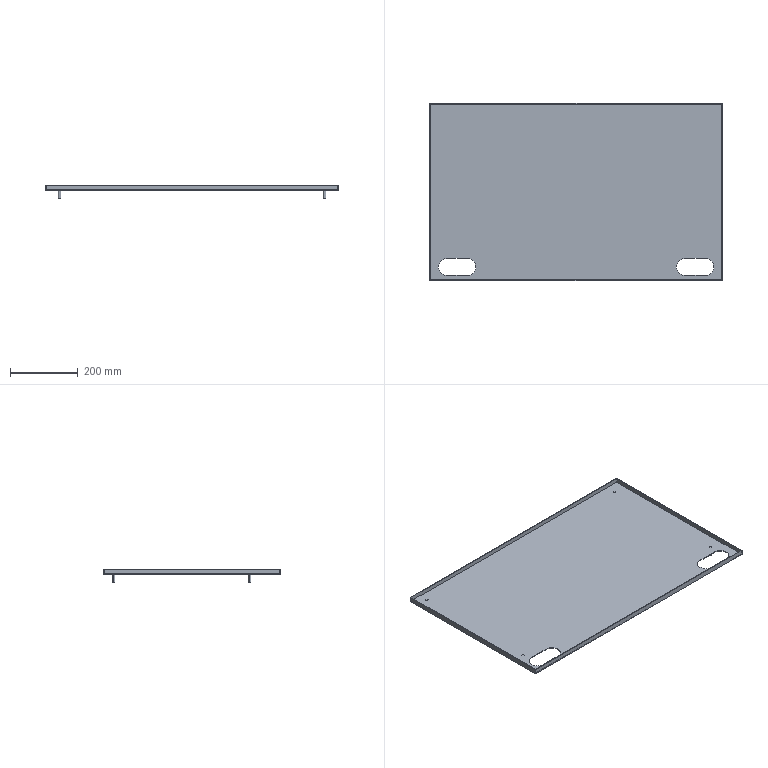Part | STEP file | 11-GYJJ-011-w111 | 1 solid | 33 faces | box 860 x 521 x 41 mm | volume 953098 mm3 | plane 19 | cylinder 14 | commonest cylinder face diameters 8 x8 50 x6
STEP:
#1=CARTESIAN_POINT('',(-394.,-169.5,-26.));
#2=VERTEX_POINT('',#1);
#3=CARTESIAN_POINT('',(-386.,-169.5,-26.));
#4=VERTEX_POINT('',#3);
#5=CARTESIAN_POINT('',(-390.,-169.5,-26.));
#6=DIRECTION('',(0.,0.,-1.));
#7=DIRECTION('',(-1.,0.,0.));
#8=AXIS2_PLACEMENT_3D('',#5,#6,#7);
#9=CIRCLE('',#8,4.);
#10=EDGE_CURVE('',#2,#4,#9,.T.);
#11=ORIENTED_EDGE('',*,*,#10,.F.);
#12=CARTESIAN_POINT('',(-394.,-169.5,0.));
#13=VERTEX_POINT('',#12);
#14=CARTESIAN_POINT('',(-394.,-169.5,-26.));
#15=DIRECTION('',(0.,0.,1.));
#16=VECTOR('',#15,1000.);
#17=LINE('',#14,#16);
#18=EDGE_CURVE('',#2,#13,#17,.T.);
#19=ORIENTED_EDGE('',*,*,#18,.T.);
#20=CARTESIAN_POINT('',(-386.,-169.5,0.));
#21=VERTEX_POINT('',#20);
#22=CARTESIAN_POINT('',(-390.,-169.5,0.));
#23=DIRECTION('',(0.,0.,-1.));
#24=DIRECTION('',(1.,0.,0.));
#25=AXIS2_PLACEMENT_3D('',#22,#23,#24);
#26=CIRCLE('',#25,4.);
#27=EDGE_CURVE('',#13,#21,#26,.T.);
#28=ORIENTED_EDGE('',*,*,#27,.T.);
#29=CARTESIAN_POINT('',(-386.,-169.5,-26.));
#30=DIRECTION('',(0.,0.,1.));
#31=VECTOR('',#30,1000.);
#32=LINE('',#29,#31);
#33=EDGE_CURVE('',#4,#21,#32,.T.);
#34=ORIENTED_EDGE('',*,*,#33,.F.);
#35=EDGE_LOOP('',(#11,#19,#28,#34));
#36=FACE_OUTER_BOUND('',#35,.T.);
#37=CARTESIAN_POINT('',(-390.,-169.5,-26.));
#38=DIRECTION('',(0.,0.,1.));
#39=DIRECTION('',(1.,0.,0.));
#40=AXIS2_PLACEMENT_3D('',#37,#38,#39);
#41=CYLINDRICAL_SURFACE('',#40,4.);
#42=ADVANCED_FACE('',(#36),#41,.T.);
#43=CARTESIAN_POINT('',(386.,-169.5,-26.));
#44=VERTEX_POINT('',#43);
#45=CARTESIAN_POINT('',(394.,-169.5,-26.));
#46=VERTEX_POINT('',#45);
#47=CARTESIAN_POINT('',(390.,-169.5,-26.));
#48=DIRECTION('',(0.,0.,-1.));
#49=DIRECTION('',(-1.,0.,0.));
#50=AXIS2_PLACEMENT_3D('',#47,#48,#49);
#51=CIRCLE('',#50,4.);
#52=EDGE_CURVE('',#44,#46,#51,.T.);
#53=ORIENTED_EDGE('',*,*,#52,.F.);
#54=CARTESIAN_POINT('',(386.,-169.5,0.));
#55=VERTEX_POINT('',#54);
#56=CARTESIAN_POINT('',(386.,-169.5,-26.));
#57=DIRECTION('',(0.,0.,1.));
#58=VECTOR('',#57,1000.);
#59=LINE('',#56,#58);
#60=EDGE_CURVE('',#44,#55,#59,.T.);
#61=ORIENTED_EDGE('',*,*,#60,.T.);
#62=CARTESIAN_POINT('',(394.,-169.5,0.));
#63=VERTEX_POINT('',#62);
#64=CARTESIAN_POINT('',(390.,-169.5,0.));
#65=DIRECTION('',(0.,0.,-1.));
#66=DIRECTION('',(1.,0.,0.));
#67=AXIS2_PLACEMENT_3D('',#64,#65,#66);
#68=CIRCLE('',#67,4.);
#69=EDGE_CURVE('',#55,#63,#68,.T.);
#70=ORIENTED_EDGE('',*,*,#69,.T.);
#71=CARTESIAN_POINT('',(394.,-169.5,-26.));
#72=DIRECTION('',(0.,0.,1.));
#73=VECTOR('',#72,1000.);
#74=LINE('',#71,#73);
#75=EDGE_CURVE('',#46,#63,#74,.T.);
#76=ORIENTED_EDGE('',*,*,#75,.F.);
#77=EDGE_LOOP('',(#53,#61,#70,#76));
#78=FACE_OUTER_BOUND('',#77,.T.);
#79=CARTESIAN_POINT('',(390.,-169.5,-26.));
#80=DIRECTION('',(0.,0.,1.));
#81=DIRECTION('',(1.,0.,0.));
#82=AXIS2_PLACEMENT_3D('',#79,#80,#81);
#83=CYLINDRICAL_SURFACE('',#82,4.);
#84=ADVANCED_FACE('',(#78),#83,.T.);
#85=CARTESIAN_POINT('',(-394.,230.5,-26.));
#86=VERTEX_POINT('',#85);
#87=CARTESIAN_POINT('',(-386.,230.5,-26.));
#88=VERTEX_POINT('',#87);
#89=CARTESIAN_POINT('',(-390.,230.5,-26.));
#90=DIRECTION('',(0.,0.,-1.));
#91=DIRECTION('',(-1.,0.,0.));
#92=AXIS2_PLACEMENT_3D('',#89,#90,#91);
#93=CIRCLE('',#92,4.);
#94=EDGE_CURVE('',#86,#88,#93,.T.);
#95=ORIENTED_EDGE('',*,*,#94,.F.);
#96=CARTESIAN_POINT('',(-394.,230.5,0.));
#97=VERTEX_POINT('',#96);
#98=CARTESIAN_POINT('',(-394.,230.5,-26.));
#99=DIRECTION('',(0.,0.,1.));
#100=VECTOR('',#99,1000.);
#101=LINE('',#98,#100);
#102=EDGE_CURVE('',#86,#97,#101,.T.);
#103=ORIENTED_EDGE('',*,*,#102,.T.);
#104=CARTESIAN_POINT('',(-386.,230.5,0.));
#105=VERTEX_POINT('',#104);
#106=CARTESIAN_POINT('',(-390.,230.5,0.));
#107=DIRECTION('',(0.,0.,-1.));
#108=DIRECTION('',(1.,0.,0.));
#109=AXIS2_PLACEMENT_3D('',#106,#107,#108);
#110=CIRCLE('',#109,4.);
#111=EDGE_CURVE('',#97,#105,#110,.T.);
#112=ORIENTED_EDGE('',*,*,#111,.T.);
#113=CARTESIAN_POINT('',(-386.,230.5,-26.));
#114=DIRECTION('',(0.,0.,1.));
#115=VECTOR('',#114,1000.);
#116=LINE('',#113,#115);
#117=EDGE_CURVE('',#88,#105,#116,.T.);
#118=ORIENTED_EDGE('',*,*,#117,.F.);
#119=EDGE_LOOP('',(#95,#103,#112,#118));
#120=FACE_OUTER_BOUND('',#119,.T.);
#121=CARTESIAN_POINT('',(-390.,230.5,-26.));
#122=DIRECTION('',(0.,0.,1.));
#123=DIRECTION('',(1.,0.,0.));
#124=AXIS2_PLACEMENT_3D('',#121,#122,#123);
#125=CYLINDRICAL_SURFACE('',#124,4.);
#126=ADVANCED_FACE('',(#120),#125,.T.);
#127=CARTESIAN_POINT('',(386.,230.5,-26.));
#128=VERTEX_POINT('',#127);
#129=CARTESIAN_POINT('',(394.,230.5,-26.));
#130=VERTEX_POINT('',#129);
#131=CARTESIAN_POINT('',(390.,230.5,-26.));
#132=DIRECTION('',(0.,0.,-1.));
#133=DIRECTION('',(-1.,0.,0.));
#134=AXIS2_PLACEMENT_3D('',#131,#132,#133);
#135=CIRCLE('',#134,4.);
#136=EDGE_CURVE('',#128,#130,#135,.T.);
#137=ORIENTED_EDGE('',*,*,#136,.F.);
#138=CARTESIAN_POINT('',(386.,230.5,0.));
#139=VERTEX_POINT('',#138);
#140=CARTESIAN_POINT('',(386.,230.5,-26.));
#141=DIRECTION('',(0.,0.,1.));
#142=VECTOR('',#141,1000.);
#143=LINE('',#140,#142);
#144=EDGE_CURVE('',#128,#139,#143,.T.);
#145=ORIENTED_EDGE('',*,*,#144,.T.);
#146=CARTESIAN_POINT('',(394.,230.5,0.));
#147=VERTEX_POINT('',#146);
#148=CARTESIAN_POINT('',(390.,230.5,0.));
#149=DIRECTION('',(0.,0.,-1.));
#150=DIRECTION('',(1.,0.,0.));
#151=AXIS2_PLACEMENT_3D('',#148,#149,#150);
#152=CIRCLE('',#151,4.);
#153=EDGE_CURVE('',#139,#147,#152,.T.);
#154=ORIENTED_EDGE('',*,*,#153,.T.);
#155=CARTESIAN_POINT('',(394.,230.5,-26.));
#156=DIRECTION('',(0.,0.,1.));
#157=VECTOR('',#156,1000.);
#158=LINE('',#155,#157);
#159=EDGE_CURVE('',#130,#147,#158,.T.);
#160=ORIENTED_EDGE('',*,*,#159,.F.);
#161=EDGE_LOOP('',(#137,#145,#154,#160));
#162=FACE_OUTER_BOUND('',#161,.T.);
#163=CARTESIAN_POINT('',(390.,230.5,-26.));
#164=DIRECTION('',(0.,0.,1.));
#165=DIRECTION('',(1.,0.,0.));
#166=AXIS2_PLACEMENT_3D('',#163,#164,#165);
#167=CYLINDRICAL_SURFACE('',#166,4.);
#168=ADVANCED_FACE('',(#162),#167,.T.);
#169=CARTESIAN_POINT('',(-405.,-220.5,2.));
#170=VERTEX_POINT('',#169);
#171=CARTESIAN_POINT('',(-380.,-195.5,2.));
#172=VERTEX_POINT('',#171);
#173=CARTESIAN_POINT('',(-380.,-220.5,2.));
#174=DIRECTION('',(0.,0.,-1.));
#175=DIRECTION('',(1.,0.,0.));
#176=AXIS2_PLACEMENT_3D('',#173,#174,#175);
#177=CIRCLE('',#176,25.);
#178=EDGE_CURVE('',#170,#172,#177,.T.);
#179=ORIENTED_EDGE('',*,*,#178,.F.);
#180=CARTESIAN_POINT('',(-405.,-220.5,0.));
#181=VERTEX_POINT('',#180);
#182=CARTESIAN_POINT('',(-405.,-220.5,10.));
#183=DIRECTION('',(0.,0.,-1.));
#184=VECTOR('',#183,1000.);
#185=LINE('',#182,#184);
#186=EDGE_CURVE('',#170,#181,#185,.T.);
#187=ORIENTED_EDGE('',*,*,#186,.T.);
#188=CARTESIAN_POINT('',(-380.,-195.5,0.));
#189=VERTEX_POINT('',#188);
#190=CARTESIAN_POINT('',(-380.,-220.5,0.));
#191=DIRECTION('',(0.,0.,1.));
#192=DIRECTION('',(1.,0.,0.));
#193=AXIS2_PLACEMENT_3D('',#190,#191,#192);
#194=CIRCLE('',#193,25.);
#195=EDGE_CURVE('',#189,#181,#194,.T.);
#196=ORIENTED_EDGE('',*,*,#195,.F.);
#197=CARTESIAN_POINT('',(-380.,-195.5,10.));
#198=DIRECTION('',(0.,0.,-1.));
#199=VECTOR('',#198,1000.);
#200=LINE('',#197,#199);
#201=EDGE_CURVE('',#172,#189,#200,.T.);
#202=ORIENTED_EDGE('',*,*,#201,.F.);
#203=EDGE_LOOP('',(#179,#187,#196,#202));
#204=FACE_OUTER_BOUND('',#203,.T.);
#205=CARTESIAN_POINT('',(-380.,-220.5,10.));
#206=DIRECTION('',(0.,0.,-1.));
#207=DIRECTION('',(-1.,0.,0.));
#208=AXIS2_PLACEMENT_3D('',#205,#206,#207);
#209=CYLINDRICAL_SURFACE('',#208,25.);
#210=ADVANCED_FACE('',(#204),#209,.F.);
#211=CARTESIAN_POINT('',(320.,-195.5,2.));
#212=VERTEX_POINT('',#211);
#213=CARTESIAN_POINT('',(295.,-220.5,2.));
#214=VERTEX_POINT('',#213);
#215=CARTESIAN_POINT('',(320.,-220.5,2.));
#216=DIRECTION('',(0.,0.,1.));
#217=DIRECTION('',(1.,0.,0.));
#218=AXIS2_PLACEMENT_3D('',#215,#216,#217);
#219=CIRCLE('',#218,25.);
#220=EDGE_CURVE('',#212,#214,#219,.T.);
#221=ORIENTED_EDGE('',*,*,#220,.T.);
#222=CARTESIAN_POINT('',(295.,-220.5,0.));
#223=VERTEX_POINT('',#222);
#224=CARTESIAN_POINT('',(295.,-220.5,10.));
#225=DIRECTION('',(0.,0.,-1.));
#226=VECTOR('',#225,1000.);
#227=LINE('',#224,#226);
#228=EDGE_CURVE('',#214,#223,#227,.T.);
#229=ORIENTED_EDGE('',*,*,#228,.T.);
#230=CARTESIAN_POINT('',(320.,-195.5,0.));
#231=VERTEX_POINT('',#230);
#232=CARTESIAN_POINT('',(320.,-220.5,0.));
#233=DIRECTION('',(0.,0.,-1.));
#234=DIRECTION('',(-1.,0.,0.));
#235=AXIS2_PLACEMENT_3D('',#232,#233,#234);
#236=CIRCLE('',#235,25.);
#237=EDGE_CURVE('',#223,#231,#236,.T.);
#238=ORIENTED_EDGE('',*,*,#237,.T.);
#239=CARTESIAN_POINT('',(320.,-195.5,10.));
#240=DIRECTION('',(0.,0.,-1.));
#241=VECTOR('',#240,1000.);
#242=LINE('',#239,#241);
#243=EDGE_CURVE('',#212,#231,#242,.T.);
#244=ORIENTED_EDGE('',*,*,#243,.F.);
#245=EDGE_LOOP('',(#221,#229,#238,#244));
#246=FACE_OUTER_BOUND('',#245,.T.);
#247=CARTESIAN_POINT('',(320.,-220.5,10.));
#248=DIRECTION('',(0.,0.,-1.));
#249=DIRECTION('',(-1.,0.,0.));
#250=AXIS2_PLACEMENT_3D('',#247,#248,#249);
#251=CYLINDRICAL_SURFACE('',#250,25.);
#252=ADVANCED_FACE('',(#246),#251,.F.);
#253=CARTESIAN_POINT('',(-390.,-169.5,0.));
#254=DIRECTION('',(0.,0.,-1.));
#255=DIRECTION('',(1.,0.,0.));
#256=AXIS2_PLACEMENT_3D('',#253,#254,#255);
#257=CIRCLE('',#256,4.);
#258=EDGE_CURVE('',#21,#13,#257,.T.);
#259=ORIENTED_EDGE('',*,*,#258,.F.);
#260=ORIENTED_EDGE('',*,*,#27,.F.);
#261=EDGE_LOOP('',(#259,#260));
#262=FACE_BOUND('',#261,.T.);
#263=CARTESIAN_POINT('',(390.,-169.5,0.));
#264=DIRECTION('',(0.,0.,-1.));
#265=DIRECTION('',(1.,0.,0.));
#266=AXIS2_PLACEMENT_3D('',#263,#264,#265);
#267=CIRCLE('',#266,4.);
#268=EDGE_CURVE('',#63,#55,#267,.T.);
#269=ORIENTED_EDGE('',*,*,#268,.F.);
#270=ORIENTED_EDGE('',*,*,#69,.F.);
#271=EDGE_LOOP('',(#269,#270));
#272=FACE_BOUND('',#271,.T.);
#273=CARTESIAN_POINT('',(-390.,230.5,0.));
#274=DIRECTION('',(0.,0.,-1.));
#275=DIRECTION('',(1.,0.,0.));
#276=AXIS2_PLACEMENT_3D('',#273,#274,#275);
#277=CIRCLE('',#276,4.);
#278=EDGE_CURVE('',#105,#97,#277,.T.);
#279=ORIENTED_EDGE('',*,*,#278,.F.);
#280=ORIENTED_EDGE('',*,*,#111,.F.);
#281=EDGE_LOOP('',(#279,#280));
#282=FACE_BOUND('',#281,.T.);
#283=CARTESIAN_POINT('',(390.,230.5,0.));
#284=DIRECTION('',(0.,0.,-1.));
#285=DIRECTION('',(1.,0.,0.));
#286=AXIS2_PLACEMENT_3D('',#283,#284,#285);
#287=CIRCLE('',#286,4.);
#288=EDGE_CURVE('',#147,#139,#287,.T.);
#289=ORIENTED_EDGE('',*,*,#288,.F.);
#290=ORIENTED_EDGE('',*,*,#153,.F.);
#291=EDGE_LOOP('',(#289,#290));
#292=FACE_BOUND('',#291,.T.);
#293=CARTESIAN_POINT('',(430.,-260.5,0.));
#294=VERTEX_POINT('',#293);
#295=CARTESIAN_POINT('',(430.,260.5,0.));
#296=VERTEX_POINT('',#295);
#297=CARTESIAN_POINT('',(430.,260.5,0.));
#298=DIRECTION('',(0.,1.,0.));
#299=VECTOR('',#298,1000.);
#300=LINE('',#297,#299);
#301=EDGE_CURVE('',#294,#296,#300,.T.);
#302=ORIENTED_EDGE('',*,*,#301,.F.);
#303=CARTESIAN_POINT('',(-430.,-260.5,0.));
#304=VERTEX_POINT('',#303);
#305=CARTESIAN_POINT('',(-430.,-260.5,0.));
#306=DIRECTION('',(1.,0.,0.));
#307=VECTOR('',#306,1000.);
#308=LINE('',#305,#307);
#309=EDGE_CURVE('',#304,#294,#308,.T.);
#310=ORIENTED_EDGE('',*,*,#309,.F.);
#311=CARTESIAN_POINT('',(-430.,260.5,0.));
#312=VERTEX_POINT('',#311);
#313=CARTESIAN_POINT('',(-430.,260.5,0.));
#314=DIRECTION('',(0.,-1.,0.));
#315=VECTOR('',#314,1000.);
#316=LINE('',#313,#315);
#317=EDGE_CURVE('',#312,#304,#316,.T.);
#318=ORIENTED_EDGE('',*,*,#317,.F.);
#319=CARTESIAN_POINT('',(-430.,260.5,0.));
#320=DIRECTION('',(-1.,0.,0.));
#321=VECTOR('',#320,1000.);
#322=LINE('',#319,#321);
#323=EDGE_CURVE('',#296,#312,#322,.T.);
#324=ORIENTED_EDGE('',*,*,#323,.F.);
#325=EDGE_LOOP('',(#302,#310,#318,#324));
#326=FACE_OUTER_BOUND('',#325,.T.);
#327=CARTESIAN_POINT('',(380.,-245.5,0.));
#328=VERTEX_POINT('',#327);
#329=CARTESIAN_POINT('',(320.,-245.5,0.));
#330=VERTEX_POINT('',#329);
#331=CARTESIAN_POINT('',(380.,-245.5,0.));
#332=DIRECTION('',(-1.,0.,0.));
#333=VECTOR('',#332,1000.);
#334=LINE('',#331,#333);
#335=EDGE_CURVE('',#328,#330,#334,.T.);
#336=ORIENTED_EDGE('',*,*,#335,.F.);
#337=CARTESIAN_POINT('',(380.,-195.5,0.));
#338=VERTEX_POINT('',#337);
#339=CARTESIAN_POINT('',(380.,-220.5,0.));
#340=DIRECTION('',(0.,0.,-1.));
#341=DIRECTION('',(-1.,0.,0.));
#342=AXIS2_PLACEMENT_3D('',#339,#340,#341);
#343=CIRCLE('',#342,25.);
#344=EDGE_CURVE('',#338,#328,#343,.T.);
#345=ORIENTED_EDGE('',*,*,#344,.F.);
#346=CARTESIAN_POINT('',(380.,-195.5,0.));
#347=DIRECTION('',(1.,0.,0.));
#348=VECTOR('',#347,1000.);
#349=LINE('',#346,#348);
#350=EDGE_CURVE('',#231,#338,#349,.T.);
#351=ORIENTED_EDGE('',*,*,#350,.F.);
#352=ORIENTED_EDGE('',*,*,#237,.F.);
#353=CARTESIAN_POINT('',(320.,-220.5,0.));
#354=DIRECTION('',(0.,0.,-1.));
#355=DIRECTION('',(-1.,0.,0.));
#356=AXIS2_PLACEMENT_3D('',#353,#354,#355);
#357=CIRCLE('',#356,25.);
#358=EDGE_CURVE('',#330,#223,#357,.T.);
#359=ORIENTED_EDGE('',*,*,#358,.F.);
#360=EDGE_LOOP('',(#336,#345,#351,#352,#359));
#361=FACE_BOUND('',#360,.T.);
#362=ORIENTED_EDGE('',*,*,#195,.T.);
#363=CARTESIAN_POINT('',(-380.,-245.5,0.));
#364=VERTEX_POINT('',#363);
#365=CARTESIAN_POINT('',(-380.,-220.5,0.));
#366=DIRECTION('',(0.,0.,1.));
#367=DIRECTION('',(1.,0.,0.));
#368=AXIS2_PLACEMENT_3D('',#365,#366,#367);
#369=CIRCLE('',#368,25.);
#370=EDGE_CURVE('',#181,#364,#369,.T.);
#371=ORIENTED_EDGE('',*,*,#370,.T.);
#372=CARTESIAN_POINT('',(-320.,-245.5,0.));
#373=VERTEX_POINT('',#372);
#374=CARTESIAN_POINT('',(-380.,-245.5,0.));
#375=DIRECTION('',(1.,0.,0.));
#376=VECTOR('',#375,1000.);
#377=LINE('',#374,#376);
#378=EDGE_CURVE('',#364,#373,#377,.T.);
#379=ORIENTED_EDGE('',*,*,#378,.T.);
#380=CARTESIAN_POINT('',(-320.,-195.5,0.));
#381=VERTEX_POINT('',#380);
#382=CARTESIAN_POINT('',(-320.,-220.5,0.));
#383=DIRECTION('',(0.,0.,1.));
#384=DIRECTION('',(1.,0.,0.));
#385=AXIS2_PLACEMENT_3D('',#382,#383,#384);
#386=CIRCLE('',#385,25.);
#387=EDGE_CURVE('',#373,#381,#386,.T.);
#388=ORIENTED_EDGE('',*,*,#387,.T.);
#389=CARTESIAN_POINT('',(-380.,-195.5,0.));
#390=DIRECTION('',(-1.,0.,0.));
#391=VECTOR('',#390,1000.);
#392=LINE('',#389,#391);
#393=EDGE_CURVE('',#381,#189,#392,.T.);
#394=ORIENTED_EDGE('',*,*,#393,.T.);
#395=EDGE_LOOP('',(#362,#371,#379,#388,#394));
#396=FACE_BOUND('',#395,.T.);
#397=CARTESIAN_POINT('',(0.,0.,0.));
#398=DIRECTION('',(0.,0.,1.));
#399=DIRECTION('',(1.,0.,0.));
#400=AXIS2_PLACEMENT_3D('',#397,#398,#399);
#401=PLANE('',#400);
#402=ADVANCED_FACE('',(#262,#272,#282,#292,#326,#361,#396),#401,.F.);
#403=CARTESIAN_POINT('',(380.,-245.5,2.));
#404=VERTEX_POINT('',#403);
#405=CARTESIAN_POINT('',(380.,-195.5,2.));
#406=VERTEX_POINT('',#405);
#407=CARTESIAN_POINT('',(380.,-220.5,2.));
#408=DIRECTION('',(0.,0.,1.));
#409=DIRECTION('',(1.,0.,0.));
#410=AXIS2_PLACEMENT_3D('',#407,#408,#409);
#411=CIRCLE('',#410,25.);
#412=EDGE_CURVE('',#404,#406,#411,.T.);
#413=ORIENTED_EDGE('',*,*,#412,.F.);
#414=CARTESIAN_POINT('',(320.,-245.5,2.));
#415=VERTEX_POINT('',#414);
#416=CARTESIAN_POINT('',(0.,-245.5,2.));
#417=DIRECTION('',(1.,0.,0.));
#418=VECTOR('',#417,1000.);
#419=LINE('',#416,#418);
#420=EDGE_CURVE('',#415,#404,#419,.T.);
#421=ORIENTED_EDGE('',*,*,#420,.F.);
#422=CARTESIAN_POINT('',(320.,-220.5,2.));
#423=DIRECTION('',(0.,0.,1.));
#424=DIRECTION('',(1.,0.,0.));
#425=AXIS2_PLACEMENT_3D('',#422,#423,#424);
#426=CIRCLE('',#425,25.);
#427=EDGE_CURVE('',#214,#415,#426,.T.);
#428=ORIENTED_EDGE('',*,*,#427,.F.);
#429=ORIENTED_EDGE('',*,*,#220,.F.);
#430=CARTESIAN_POINT('',(0.,-195.5,2.));
#431=DIRECTION('',(-1.,0.,0.));
#432=VECTOR('',#431,1000.);
#433=LINE('',#430,#432);
#434=EDGE_CURVE('',#406,#212,#433,.T.);
#435=ORIENTED_EDGE('',*,*,#434,.F.);
#436=EDGE_LOOP('',(#413,#421,#428,#429,#435));
#437=FACE_BOUND('',#436,.T.);
#438=CARTESIAN_POINT('',(428.,-258.5,2.));
#439=VERTEX_POINT('',#438);
#440=CARTESIAN_POINT('',(428.,258.5,2.));
#441=VERTEX_POINT('',#440);
#442=CARTESIAN_POINT('',(428.,260.5,2.));
#443=DIRECTION('',(0.,1.,0.));
#444=VECTOR('',#443,1000.);
#445=LINE('',#442,#444);
#446=EDGE_CURVE('',#439,#441,#445,.T.);
#447=ORIENTED_EDGE('',*,*,#446,.T.);
#448=CARTESIAN_POINT('',(-428.,258.5,2.));
#449=VERTEX_POINT('',#448);
#450=CARTESIAN_POINT('',(-430.,258.5,2.));
#451=DIRECTION('',(-1.,0.,0.));
#452=VECTOR('',#451,1000.);
#453=LINE('',#450,#452);
#454=EDGE_CURVE('',#441,#449,#453,.T.);
#455=ORIENTED_EDGE('',*,*,#454,.T.);
#456=CARTESIAN_POINT('',(-428.,-258.5,2.));
#457=VERTEX_POINT('',#456);
#458=CARTESIAN_POINT('',(-428.,260.5,2.));
#459=DIRECTION('',(0.,-1.,0.));
#460=VECTOR('',#459,1000.);
#461=LINE('',#458,#460);
#462=EDGE_CURVE('',#449,#457,#461,.T.);
#463=ORIENTED_EDGE('',*,*,#462,.T.);
#464=CARTESIAN_POINT('',(-430.,-258.5,2.));
#465=DIRECTION('',(1.,0.,0.));
#466=VECTOR('',#465,1000.);
#467=LINE('',#464,#466);
#468=EDGE_CURVE('',#457,#439,#467,.T.);
#469=ORIENTED_EDGE('',*,*,#468,.T.);
#470=EDGE_LOOP('',(#447,#455,#463,#469));
#471=FACE_OUTER_BOUND('',#470,.T.);
#472=CARTESIAN_POINT('',(-320.,-245.5,2.));
#473=VERTEX_POINT('',#472);
#474=CARTESIAN_POINT('',(-380.,-245.5,2.));
#475=VERTEX_POINT('',#474);
#476=CARTESIAN_POINT('',(0.,-245.5,2.));
#477=DIRECTION('',(-1.,0.,0.));
#478=VECTOR('',#477,1000.);
#479=LINE('',#476,#478);
#480=EDGE_CURVE('',#473,#475,#479,.T.);
#481=ORIENTED_EDGE('',*,*,#480,.T.);
#482=CARTESIAN_POINT('',(-380.,-220.5,2.));
#483=DIRECTION('',(0.,0.,-1.));
#484=DIRECTION('',(1.,0.,0.));
#485=AXIS2_PLACEMENT_3D('',#482,#483,#484);
#486=CIRCLE('',#485,25.);
#487=EDGE_CURVE('',#475,#170,#486,.T.);
#488=ORIENTED_EDGE('',*,*,#487,.T.);
#489=ORIENTED_EDGE('',*,*,#178,.T.);
#490=CARTESIAN_POINT('',(-320.,-195.5,2.));
#491=VERTEX_POINT('',#490);
#492=CARTESIAN_POINT('',(0.,-195.5,2.));
#493=DIRECTION('',(1.,0.,0.));
#494=VECTOR('',#493,1000.);
#495=LINE('',#492,#494);
#496=EDGE_CURVE('',#172,#491,#495,.T.);
#497=ORIENTED_EDGE('',*,*,#496,.T.);
#498=CARTESIAN_POINT('',(-320.,-220.5,2.));
#499=DIRECTION('',(0.,0.,-1.));
#500=DIRECTION('',(1.,0.,0.));
#501=AXIS2_PLACEMENT_3D('',#498,#499,#500);
#502=CIRCLE('',#501,25.);
#503=EDGE_CURVE('',#491,#473,#502,.T.);
#504=ORIENTED_EDGE('',*,*,#503,.T.);
#505=EDGE_LOOP('',(#481,#488,#489,#497,#504));
#506=FACE_BOUND('',#505,.T.);
#507=CARTESIAN_POINT('',(0.,0.,2.));
#508=DIRECTION('',(0.,0.,1.));
#509=DIRECTION('',(1.,0.,0.));
#510=AXIS2_PLACEMENT_3D('',#507,#508,#509);
#511=PLANE('',#510);
#512=ADVANCED_FACE('',(#437,#471,#506),#511,.T.);
#513=ORIENTED_EDGE('',*,*,#301,.T.);
#514=CARTESIAN_POINT('',(430.,260.5,15.));
#515=VERTEX_POINT('',#514);
#516=CARTESIAN_POINT('',(430.,260.5,15.));
#517=DIRECTION('',(0.,0.,-1.));
#518=VECTOR('',#517,1000.);
#519=LINE('',#516,#518);
#520=EDGE_CURVE('',#515,#296,#519,.T.);
#521=ORIENTED_EDGE('',*,*,#520,.F.);
#522=CARTESIAN_POINT('',(430.,-260.5,15.));
#523=VERTEX_POINT('',#522);
#524=CARTESIAN_POINT('',(430.,260.5,15.));
#525=DIRECTION('',(0.,1.,0.));
#526=VECTOR('',#525,1000.);
#527=LINE('',#524,#526);
#528=EDGE_CURVE('',#523,#515,#527,.T.);
#529=ORIENTED_EDGE('',*,*,#528,.F.);
#530=CARTESIAN_POINT('',(430.,-260.5,15.));
#531=DIRECTION('',(0.,0.,-1.));
#532=VECTOR('',#531,1000.);
#533=LINE('',#530,#532);
#534=EDGE_CURVE('',#523,#294,#533,.T.);
#535=ORIENTED_EDGE('',*,*,#534,.T.);
#536=EDGE_LOOP('',(#513,#521,#529,#535));
#537=FACE_OUTER_BOUND('',#536,.T.);
#538=CARTESIAN_POINT('',(430.,260.5,15.));
#539=DIRECTION('',(-1.,0.,0.));
#540=DIRECTION('',(0.,-1.,0.));
#541=AXIS2_PLACEMENT_3D('',#538,#539,#540);
#542=PLANE('',#541);
#543=ADVANCED_FACE('',(#537),#542,.F.);
#544=ORIENTED_EDGE('',*,*,#323,.T.);
#545=CARTESIAN_POINT('',(-430.,260.5,15.));
#546=VERTEX_POINT('',#545);
#547=CARTESIAN_POINT('',(-430.,260.5,15.));
#548=DIRECTION('',(0.,0.,-1.));
#549=VECTOR('',#548,1000.);
#550=LINE('',#547,#549);
#551=EDGE_CURVE('',#546,#312,#550,.T.);
#552=ORIENTED_EDGE('',*,*,#551,.F.);
#553=CARTESIAN_POINT('',(-430.,260.5,15.));
#554=DIRECTION('',(-1.,0.,0.));
#555=VECTOR('',#554,1000.);
#556=LINE('',#553,#555);
#557=EDGE_CURVE('',#515,#546,#556,.T.);
#558=ORIENTED_EDGE('',*,*,#557,.F.);
#559=ORIENTED_EDGE('',*,*,#520,.T.);
#560=EDGE_LOOP('',(#544,#552,#558,#559));
#561=FACE_OUTER_BOUND('',#560,.T.);
#562=CARTESIAN_POINT('',(-430.,260.5,15.));
#563=DIRECTION('',(0.,-1.,0.));
#564=DIRECTION('',(0.,0.,-1.));
#565=AXIS2_PLACEMENT_3D('',#562,#563,#564);
#566=PLANE('',#565);
#567=ADVANCED_FACE('',(#561),#566,.F.);
#568=ORIENTED_EDGE('',*,*,#317,.T.);
#569=CARTESIAN_POINT('',(-430.,-260.5,15.));
#570=VERTEX_POINT('',#569);
#571=CARTESIAN_POINT('',(-430.,-260.5,15.));
#572=DIRECTION('',(0.,0.,-1.));
#573=VECTOR('',#572,1000.);
#574=LINE('',#571,#573);
#575=EDGE_CURVE('',#570,#304,#574,.T.);
#576=ORIENTED_EDGE('',*,*,#575,.F.);
#577=CARTESIAN_POINT('',(-430.,260.5,15.));
#578=DIRECTION('',(0.,-1.,0.));
#579=VECTOR('',#578,1000.);
#580=LINE('',#577,#579);
#581=EDGE_CURVE('',#546,#570,#580,.T.);
#582=ORIENTED_EDGE('',*,*,#581,.F.);
#583=ORIENTED_EDGE('',*,*,#551,.T.);
#584=EDGE_LOOP('',(#568,#576,#582,#583));
#585=FACE_OUTER_BOUND('',#584,.T.);
#586=CARTESIAN_POINT('',(-430.,260.5,15.));
#587=DIRECTION('',(1.,0.,0.));
#588=DIRECTION('',(0.,0.,-1.));
#589=AXIS2_PLACEMENT_3D('',#586,#587,#588);
#590=PLANE('',#589);
#591=ADVANCED_FACE('',(#585),#590,.F.);
#592=ORIENTED_EDGE('',*,*,#309,.T.);
#593=ORIENTED_EDGE('',*,*,#534,.F.);
#594=CARTESIAN_POINT('',(-430.,-260.5,15.));
#595=DIRECTION('',(1.,0.,0.));
#596=VECTOR('',#595,1000.);
#597=LINE('',#594,#596);
#598=EDGE_CURVE('',#570,#523,#597,.T.);
#599=ORIENTED_EDGE('',*,*,#598,.F.);
#600=ORIENTED_EDGE('',*,*,#575,.T.);
#601=EDGE_LOOP('',(#592,#593,#599,#600));
#602=FACE_OUTER_BOUND('',#601,.T.);
#603=CARTESIAN_POINT('',(-430.,-260.5,15.));
#604=DIRECTION('',(0.,1.,0.));
#605=DIRECTION('',(0.,0.,1.));
#606=AXIS2_PLACEMENT_3D('',#603,#604,#605);
#607=PLANE('',#606);
#608=ADVANCED_FACE('',(#602),#607,.F.);
#609=CARTESIAN_POINT('',(428.,-258.5,15.));
#610=VERTEX_POINT('',#609);
#611=CARTESIAN_POINT('',(428.,258.5,15.));
#612=VERTEX_POINT('',#611);
#613=CARTESIAN_POINT('',(428.,260.5,15.));
#614=DIRECTION('',(0.,1.,0.));
#615=VECTOR('',#614,1000.);
#616=LINE('',#613,#615);
#617=EDGE_CURVE('',#610,#612,#616,.T.);
#618=ORIENTED_EDGE('',*,*,#617,.F.);
#619=CARTESIAN_POINT('',(-428.,-258.5,15.));
#620=VERTEX_POINT('',#619);
#621=CARTESIAN_POINT('',(-430.,-258.5,15.));
#622=DIRECTION('',(1.,0.,0.));
#623=VECTOR('',#622,1000.);
#624=LINE('',#621,#623);
#625=EDGE_CURVE('',#620,#610,#624,.T.);
#626=ORIENTED_EDGE('',*,*,#625,.F.);
#627=CARTESIAN_POINT('',(-428.,258.5,15.));
#628=VERTEX_POINT('',#627);
#629=CARTESIAN_POINT('',(-428.,260.5,15.));
#630=DIRECTION('',(0.,-1.,0.));
#631=VECTOR('',#630,1000.);
#632=LINE('',#629,#631);
#633=EDGE_CURVE('',#628,#620,#632,.T.);
#634=ORIENTED_EDGE('',*,*,#633,.F.);
#635=CARTESIAN_POINT('',(-430.,258.5,15.));
#636=DIRECTION('',(-1.,0.,0.));
#637=VECTOR('',#636,1000.);
#638=LINE('',#635,#637);
#639=EDGE_CURVE('',#612,#628,#638,.T.);
#640=ORIENTED_EDGE('',*,*,#639,.F.);
#641=EDGE_LOOP('',(#618,#626,#634,#640));
#642=FACE_BOUND('',#641,.T.);
#643=ORIENTED_EDGE('',*,*,#528,.T.);
#644=ORIENTED_EDGE('',*,*,#557,.T.);
#645=ORIENTED_EDGE('',*,*,#581,.T.);
#646=ORIENTED_EDGE('',*,*,#598,.T.);
#647=EDGE_LOOP('',(#643,#644,#645,#646));
#648=FACE_OUTER_BOUND('',#647,.T.);
#649=CARTESIAN_POINT('',(0.,0.,15.));
#650=DIRECTION('',(0.,0.,1.));
#651=DIRECTION('',(1.,0.,0.));
#652=AXIS2_PLACEMENT_3D('',#649,#650,#651);
#653=PLANE('',#652);
#654=ADVANCED_FACE('',(#642,#648),#653,.T.);
#655=ORIENTED_EDGE('',*,*,#446,.F.);
#656=CARTESIAN_POINT('',(428.,-258.5,15.));
#657=DIRECTION('',(0.,0.,-1.));
#658=VECTOR('',#657,1000.);
#659=LINE('',#656,#658);
#660=EDGE_CURVE('',#610,#439,#659,.T.);
#661=ORIENTED_EDGE('',*,*,#660,.F.);
#662=ORIENTED_EDGE('',*,*,#617,.T.);
#663=CARTESIAN_POINT('',(428.,258.5,15.));
#664=DIRECTION('',(0.,0.,-1.));
#665=VECTOR('',#664,1000.);
#666=LINE('',#663,#665);
#667=EDGE_CURVE('',#612,#441,#666,.T.);
#668=ORIENTED_EDGE('',*,*,#667,.T.);
#669=EDGE_LOOP('',(#655,#661,#662,#668));
#670=FACE_OUTER_BOUND('',#669,.T.);
#671=CARTESIAN_POINT('',(428.,260.5,15.));
#672=DIRECTION('',(-1.,0.,0.));
#673=DIRECTION('',(0.,-1.,0.));
#674=AXIS2_PLACEMENT_3D('',#671,#672,#673);
#675=PLANE('',#674);
#676=ADVANCED_FACE('',(#670),#675,.T.);
#677=ORIENTED_EDGE('',*,*,#454,.F.);
#678=ORIENTED_EDGE('',*,*,#667,.F.);
#679=ORIENTED_EDGE('',*,*,#639,.T.);
#680=CARTESIAN_POINT('',(-428.,258.5,15.));
#681=DIRECTION('',(0.,0.,-1.));
#682=VECTOR('',#681,1000.);
#683=LINE('',#680,#682);
#684=EDGE_CURVE('',#628,#449,#683,.T.);
#685=ORIENTED_EDGE('',*,*,#684,.T.);
#686=EDGE_LOOP('',(#677,#678,#679,#685));
#687=FACE_OUTER_BOUND('',#686,.T.);
#688=CARTESIAN_POINT('',(-430.,258.5,15.));
#689=DIRECTION('',(0.,-1.,0.));
#690=DIRECTION('',(0.,0.,-1.));
#691=AXIS2_PLACEMENT_3D('',#688,#689,#690);
#692=PLANE('',#691);
#693=ADVANCED_FACE('',(#687),#692,.T.);
#694=ORIENTED_EDGE('',*,*,#462,.F.);
#695=ORIENTED_EDGE('',*,*,#684,.F.);
#696=ORIENTED_EDGE('',*,*,#633,.T.);
#697=CARTESIAN_POINT('',(-428.,-258.5,15.));
#698=DIRECTION('',(0.,0.,-1.));
#699=VECTOR('',#698,1000.);
#700=LINE('',#697,#699);
#701=EDGE_CURVE('',#620,#457,#700,.T.);
#702=ORIENTED_EDGE('',*,*,#701,.T.);
#703=EDGE_LOOP('',(#694,#695,#696,#702));
#704=FACE_OUTER_BOUND('',#703,.T.);
#705=CARTESIAN_POINT('',(-428.,260.5,15.));
#706=DIRECTION('',(1.,0.,0.));
#707=DIRECTION('',(0.,0.,-1.));
#708=AXIS2_PLACEMENT_3D('',#705,#706,#707);
#709=PLANE('',#708);
#710=ADVANCED_FACE('',(#704),#709,.T.);
#711=ORIENTED_EDGE('',*,*,#468,.F.);
#712=ORIENTED_EDGE('',*,*,#701,.F.);
#713=ORIENTED_EDGE('',*,*,#625,.T.);
#714=ORIENTED_EDGE('',*,*,#660,.T.);
#715=EDGE_LOOP('',(#711,#712,#713,#714));
#716=FACE_OUTER_BOUND('',#715,.T.);
#717=CARTESIAN_POINT('',(-430.,-258.5,15.));
#718=DIRECTION('',(0.,1.,0.));
#719=DIRECTION('',(0.,0.,1.));
#720=AXIS2_PLACEMENT_3D('',#717,#718,#719);
#721=PLANE('',#720);
#722=ADVANCED_FACE('',(#716),#721,.T.);
#723=ORIENTED_EDGE('',*,*,#412,.T.);
#724=CARTESIAN_POINT('',(380.,-195.5,10.));
#725=DIRECTION('',(0.,0.,-1.));
#726=VECTOR('',#725,1000.);
#727=LINE('',#724,#726);
#728=EDGE_CURVE('',#406,#338,#727,.T.);
#729=ORIENTED_EDGE('',*,*,#728,.T.);
#730=ORIENTED_EDGE('',*,*,#344,.T.);
#731=CARTESIAN_POINT('',(380.,-245.5,10.));
#732=DIRECTION('',(0.,0.,-1.));
#733=VECTOR('',#732,1000.);
#734=LINE('',#731,#733);
#735=EDGE_CURVE('',#404,#328,#734,.T.);
#736=ORIENTED_EDGE('',*,*,#735,.F.);
#737=EDGE_LOOP('',(#723,#729,#730,#736));
#738=FACE_OUTER_BOUND('',#737,.T.);
#739=CARTESIAN_POINT('',(380.,-220.5,10.));
#740=DIRECTION('',(0.,0.,-1.));
#741=DIRECTION('',(-1.,0.,0.));
#742=AXIS2_PLACEMENT_3D('',#739,#740,#741);
#743=CYLINDRICAL_SURFACE('',#742,25.);
#744=ADVANCED_FACE('',(#738),#743,.F.);
#745=ORIENTED_EDGE('',*,*,#434,.T.);
#746=ORIENTED_EDGE('',*,*,#243,.T.);
#747=ORIENTED_EDGE('',*,*,#350,.T.);
#748=ORIENTED_EDGE('',*,*,#728,.F.);
#749=EDGE_LOOP('',(#745,#746,#747,#748));
#750=FACE_OUTER_BOUND('',#749,.T.);
#751=CARTESIAN_POINT('',(380.,-195.5,10.));
#752=DIRECTION('',(0.,1.,0.));
#753=DIRECTION('',(0.,0.,1.));
#754=AXIS2_PLACEMENT_3D('',#751,#752,#753);
#755=PLANE('',#754);
#756=ADVANCED_FACE('',(#750),#755,.F.);
#757=ORIENTED_EDGE('',*,*,#228,.F.);
#758=ORIENTED_EDGE('',*,*,#427,.T.);
#759=CARTESIAN_POINT('',(320.,-245.5,10.));
#760=DIRECTION('',(0.,0.,-1.));
#761=VECTOR('',#760,1000.);
#762=LINE('',#759,#761);
#763=EDGE_CURVE('',#415,#330,#762,.T.);
#764=ORIENTED_EDGE('',*,*,#763,.T.);
#765=ORIENTED_EDGE('',*,*,#358,.T.);
#766=EDGE_LOOP('',(#757,#758,#764,#765));
#767=FACE_OUTER_BOUND('',#766,.T.);
#768=CARTESIAN_POINT('',(320.,-220.5,10.));
#769=DIRECTION('',(0.,0.,-1.));
#770=DIRECTION('',(-1.,0.,0.));
#771=AXIS2_PLACEMENT_3D('',#768,#769,#770);
#772=CYLINDRICAL_SURFACE('',#771,25.);
#773=ADVANCED_FACE('',(#767),#772,.F.);
#774=ORIENTED_EDGE('',*,*,#420,.T.);
#775=ORIENTED_EDGE('',*,*,#735,.T.);
#776=ORIENTED_EDGE('',*,*,#335,.T.);
#777=ORIENTED_EDGE('',*,*,#763,.F.);
#778=EDGE_LOOP('',(#774,#775,#776,#777));
#779=FACE_OUTER_BOUND('',#778,.T.);
#780=CARTESIAN_POINT('',(380.,-245.5,10.));
#781=DIRECTION('',(0.,-1.,0.));
#782=DIRECTION('',(0.,0.,-1.));
#783=AXIS2_PLACEMENT_3D('',#780,#781,#782);
#784=PLANE('',#783);
#785=ADVANCED_FACE('',(#779),#784,.F.);
#786=ORIENTED_EDGE('',*,*,#186,.F.);
#787=ORIENTED_EDGE('',*,*,#487,.F.);
#788=CARTESIAN_POINT('',(-380.,-245.5,10.));
#789=DIRECTION('',(0.,0.,-1.));
#790=VECTOR('',#789,1000.);
#791=LINE('',#788,#790);
#792=EDGE_CURVE('',#475,#364,#791,.T.);
#793=ORIENTED_EDGE('',*,*,#792,.T.);
#794=ORIENTED_EDGE('',*,*,#370,.F.);
#795=EDGE_LOOP('',(#786,#787,#793,#794));
#796=FACE_OUTER_BOUND('',#795,.T.);
#797=CARTESIAN_POINT('',(-380.,-220.5,10.));
#798=DIRECTION('',(0.,0.,-1.));
#799=DIRECTION('',(-1.,0.,0.));
#800=AXIS2_PLACEMENT_3D('',#797,#798,#799);
#801=CYLINDRICAL_SURFACE('',#800,25.);
#802=ADVANCED_FACE('',(#796),#801,.F.);
#803=CARTESIAN_POINT('',(-320.,-245.5,10.));
#804=DIRECTION('',(0.,0.,-1.));
#805=VECTOR('',#804,1000.);
#806=LINE('',#803,#805);
#807=EDGE_CURVE('',#473,#373,#806,.T.);
#808=ORIENTED_EDGE('',*,*,#807,.T.);
#809=ORIENTED_EDGE('',*,*,#378,.F.);
#810=ORIENTED_EDGE('',*,*,#792,.F.);
#811=ORIENTED_EDGE('',*,*,#480,.F.);
#812=EDGE_LOOP('',(#808,#809,#810,#811));
#813=FACE_OUTER_BOUND('',#812,.T.);
#814=CARTESIAN_POINT('',(-380.,-245.5,10.));
#815=DIRECTION('',(0.,1.,0.));
#816=DIRECTION('',(-1.,0.,0.));
#817=AXIS2_PLACEMENT_3D('',#814,#815,#816);
#818=PLANE('',#817);
#819=ADVANCED_FACE('',(#813),#818,.T.);
#820=CARTESIAN_POINT('',(-320.,-195.5,10.));
#821=DIRECTION('',(0.,0.,-1.));
#822=VECTOR('',#821,1000.);
#823=LINE('',#820,#822);
#824=EDGE_CURVE('',#491,#381,#823,.T.);
#825=ORIENTED_EDGE('',*,*,#824,.T.);
#826=ORIENTED_EDGE('',*,*,#387,.F.);
#827=ORIENTED_EDGE('',*,*,#807,.F.);
#828=ORIENTED_EDGE('',*,*,#503,.F.);
#829=EDGE_LOOP('',(#825,#826,#827,#828));
#830=FACE_OUTER_BOUND('',#829,.T.);
#831=CARTESIAN_POINT('',(-320.,-220.5,10.));
#832=DIRECTION('',(0.,0.,-1.));
#833=DIRECTION('',(-1.,0.,0.));
#834=AXIS2_PLACEMENT_3D('',#831,#832,#833);
#835=CYLINDRICAL_SURFACE('',#834,25.);
#836=ADVANCED_FACE('',(#830),#835,.F.);
#837=ORIENTED_EDGE('',*,*,#201,.T.);
#838=ORIENTED_EDGE('',*,*,#393,.F.);
#839=ORIENTED_EDGE('',*,*,#824,.F.);
#840=ORIENTED_EDGE('',*,*,#496,.F.);
#841=EDGE_LOOP('',(#837,#838,#839,#840));
#842=FACE_OUTER_BOUND('',#841,.T.);
#843=CARTESIAN_POINT('',(-380.,-195.5,10.));
#844=DIRECTION('',(0.,-1.,0.));
#845=DIRECTION('',(1.,0.,0.));
#846=AXIS2_PLACEMENT_3D('',#843,#844,#845);
#847=PLANE('',#846);
#848=ADVANCED_FACE('',(#842),#847,.T.);
#849=ORIENTED_EDGE('',*,*,#144,.F.);
#850=CARTESIAN_POINT('',(390.,230.5,-26.));
#851=DIRECTION('',(0.,0.,-1.));
#852=DIRECTION('',(-1.,0.,0.));
#853=AXIS2_PLACEMENT_3D('',#850,#851,#852);
#854=CIRCLE('',#853,4.);
#855=EDGE_CURVE('',#130,#128,#854,.T.);
#856=ORIENTED_EDGE('',*,*,#855,.F.);
#857=ORIENTED_EDGE('',*,*,#159,.T.);
#858=ORIENTED_EDGE('',*,*,#288,.T.);
#859=EDGE_LOOP('',(#849,#856,#857,#858));
#860=FACE_OUTER_BOUND('',#859,.T.);
#861=CARTESIAN_POINT('',(390.,230.5,-26.));
#862=DIRECTION('',(0.,0.,1.));
#863=DIRECTION('',(1.,0.,0.));
#864=AXIS2_PLACEMENT_3D('',#861,#862,#863);
#865=CYLINDRICAL_SURFACE('',#864,4.);
#866=ADVANCED_FACE('',(#860),#865,.T.);
#867=ORIENTED_EDGE('',*,*,#855,.T.);
#868=ORIENTED_EDGE('',*,*,#136,.T.);
#869=EDGE_LOOP('',(#867,#868));
#870=FACE_OUTER_BOUND('',#869,.T.);
#871=CARTESIAN_POINT('',(390.,230.5,-26.));
#872=DIRECTION('',(0.,0.,-1.));
#873=DIRECTION('',(-1.,0.,0.));
#874=AXIS2_PLACEMENT_3D('',#871,#872,#873);
#875=PLANE('',#874);
#876=ADVANCED_FACE('',(#870),#875,.T.);
#877=ORIENTED_EDGE('',*,*,#102,.F.);
#878=CARTESIAN_POINT('',(-390.,230.5,-26.));
#879=DIRECTION('',(0.,0.,-1.));
#880=DIRECTION('',(-1.,0.,0.));
#881=AXIS2_PLACEMENT_3D('',#878,#879,#880);
#882=CIRCLE('',#881,4.);
#883=EDGE_CURVE('',#88,#86,#882,.T.);
#884=ORIENTED_EDGE('',*,*,#883,.F.);
#885=ORIENTED_EDGE('',*,*,#117,.T.);
#886=ORIENTED_EDGE('',*,*,#278,.T.);
#887=EDGE_LOOP('',(#877,#884,#885,#886));
#888=FACE_OUTER_BOUND('',#887,.T.);
#889=CARTESIAN_POINT('',(-390.,230.5,-26.));
#890=DIRECTION('',(0.,0.,1.));
#891=DIRECTION('',(1.,0.,0.));
#892=AXIS2_PLACEMENT_3D('',#889,#890,#891);
#893=CYLINDRICAL_SURFACE('',#892,4.);
#894=ADVANCED_FACE('',(#888),#893,.T.);
#895=ORIENTED_EDGE('',*,*,#883,.T.);
#896=ORIENTED_EDGE('',*,*,#94,.T.);
#897=EDGE_LOOP('',(#895,#896));
#898=FACE_OUTER_BOUND('',#897,.T.);
#899=CARTESIAN_POINT('',(-390.,230.5,-26.));
#900=DIRECTION('',(0.,0.,-1.));
#901=DIRECTION('',(-1.,0.,0.));
#902=AXIS2_PLACEMENT_3D('',#899,#900,#901);
#903=PLANE('',#902);
#904=ADVANCED_FACE('',(#898),#903,.T.);
#905=ORIENTED_EDGE('',*,*,#60,.F.);
#906=CARTESIAN_POINT('',(390.,-169.5,-26.));
#907=DIRECTION('',(0.,0.,-1.));
#908=DIRECTION('',(-1.,0.,0.));
#909=AXIS2_PLACEMENT_3D('',#906,#907,#908);
#910=CIRCLE('',#909,4.);
#911=EDGE_CURVE('',#46,#44,#910,.T.);
#912=ORIENTED_EDGE('',*,*,#911,.F.);
#913=ORIENTED_EDGE('',*,*,#75,.T.);
#914=ORIENTED_EDGE('',*,*,#268,.T.);
#915=EDGE_LOOP('',(#905,#912,#913,#914));
#916=FACE_OUTER_BOUND('',#915,.T.);
#917=CARTESIAN_POINT('',(390.,-169.5,-26.));
#918=DIRECTION('',(0.,0.,1.));
#919=DIRECTION('',(1.,0.,0.));
#920=AXIS2_PLACEMENT_3D('',#917,#918,#919);
#921=CYLINDRICAL_SURFACE('',#920,4.);
#922=ADVANCED_FACE('',(#916),#921,.T.);
#923=ORIENTED_EDGE('',*,*,#911,.T.);
#924=ORIENTED_EDGE('',*,*,#52,.T.);
#925=EDGE_LOOP('',(#923,#924));
#926=FACE_OUTER_BOUND('',#925,.T.);
#927=CARTESIAN_POINT('',(390.,-169.5,-26.));
#928=DIRECTION('',(0.,0.,-1.));
#929=DIRECTION('',(-1.,0.,0.));
#930=AXIS2_PLACEMENT_3D('',#927,#928,#929);
#931=PLANE('',#930);
#932=ADVANCED_FACE('',(#926),#931,.T.);
#933=ORIENTED_EDGE('',*,*,#18,.F.);
#934=CARTESIAN_POINT('',(-390.,-169.5,-26.));
#935=DIRECTION('',(0.,0.,-1.));
#936=DIRECTION('',(-1.,0.,0.));
#937=AXIS2_PLACEMENT_3D('',#934,#935,#936);
#938=CIRCLE('',#937,4.);
#939=EDGE_CURVE('',#4,#2,#938,.T.);
#940=ORIENTED_EDGE('',*,*,#939,.F.);
#941=ORIENTED_EDGE('',*,*,#33,.T.);
#942=ORIENTED_EDGE('',*,*,#258,.T.);
#943=EDGE_LOOP('',(#933,#940,#941,#942));
#944=FACE_OUTER_BOUND('',#943,.T.);
#945=CARTESIAN_POINT('',(-390.,-169.5,-26.));
#946=DIRECTION('',(0.,0.,1.));
#947=DIRECTION('',(1.,0.,0.));
#948=AXIS2_PLACEMENT_3D('',#945,#946,#947);
#949=CYLINDRICAL_SURFACE('',#948,4.);
#950=ADVANCED_FACE('',(#944),#949,.T.);
#951=ORIENTED_EDGE('',*,*,#939,.T.);
#952=ORIENTED_EDGE('',*,*,#10,.T.);
#953=EDGE_LOOP('',(#951,#952));
#954=FACE_OUTER_BOUND('',#953,.T.);
#955=CARTESIAN_POINT('',(-390.,-169.5,-26.));
#956=DIRECTION('',(0.,0.,-1.));
#957=DIRECTION('',(-1.,0.,0.));
#958=AXIS2_PLACEMENT_3D('',#955,#956,#957);
#959=PLANE('',#958);
#960=ADVANCED_FACE('',(#954),#959,.T.);
#961=CLOSED_SHELL('',(#42,#84,#126,#168,#210,#252,#402,#512,#543,#567,#591,#608,#654,#676,#693,#710,#722,#744,#756,#773,#785,#802,#819,#836,#848,#866,#876,#894,#904,#922,#932,#950,#960));
#962=MANIFOLD_SOLID_BREP('',#961);
#963=CARTESIAN_POINT('',(0.,0.,0.));
#964=DIRECTION('',(0.,0.,1.));
#965=DIRECTION('',(1.,0.,0.));
#966=AXIS2_PLACEMENT_3D('',#963,#964,#965);
#967=(LENGTH_UNIT()NAMED_UNIT(*)SI_UNIT(.MILLI.,.METRE.));
#968=UNCERTAINTY_MEASURE_WITH_UNIT(LENGTH_MEASURE(0.00001),#967,'','');
#969=(NAMED_UNIT(*)PLANE_ANGLE_UNIT()SI_UNIT($,.RADIAN.));
#970=(NAMED_UNIT(*)SI_UNIT($,.STERADIAN.)SOLID_ANGLE_UNIT());
#971=(GEOMETRIC_REPRESENTATION_CONTEXT(3)GLOBAL_UNCERTAINTY_ASSIGNED_CONTEXT((#968))GLOBAL_UNIT_ASSIGNED_CONTEXT((#967,#969,#970))REPRESENTATION_CONTEXT('',''));
#972=ADVANCED_BREP_SHAPE_REPRESENTATION('',(#962,#966),#971);